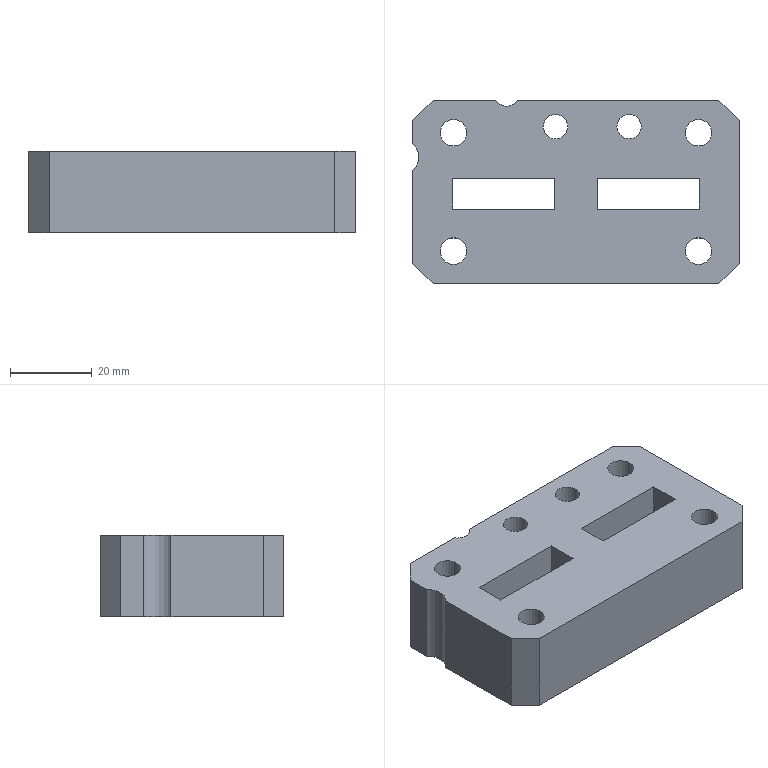Part | STEP file | P011002L003-001 | 1 solid | 36 faces | box 80 x 45 x 20 mm | volume 57856 mm3 | plane 13 | cylinder 12 | spline 11 | commonest cylinder face diameters 6.5 x4 11 x4 6 x3 9 x1